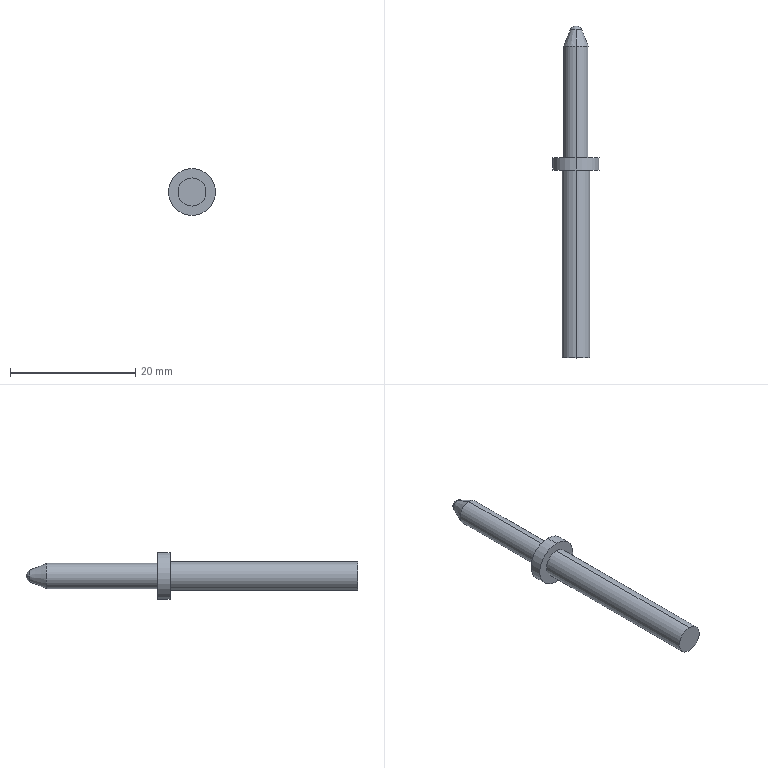Part | SolidWorks | features ICE 3, Revolution 2, Extrusion 1, RefAxis 1, RevCut 1 | 1 solid | 13 faces | box 7.5 x 53 x 7.5 mm | volume 808.158 mm3 | cylinder 6 | plane 3 | cone 2 | sphere 2 | commonest cylinder face diameters 4 x2 4.5 x2 7.5 x2
STEP:
#1=CARTESIAN_POINT('',(0.9239,20.383,0.));
#2=VERTEX_POINT('',#1);
#3=CARTESIAN_POINT('',(0.,20.383,0.9239));
#4=VERTEX_POINT('',#3);
#5=CARTESIAN_POINT('',(0.,20.383,0.));
#6=DIRECTION('',(0.,-1.,0.));
#7=DIRECTION('',(0.,0.,-1.));
#8=AXIS2_PLACEMENT_3D('',#5,#6,#7);
#9=CIRCLE('',#8,0.9239);
#10=EDGE_CURVE('',#2,#4,#9,.T.);
#11=ORIENTED_EDGE('',*,*,#10,.T.);
#12=CARTESIAN_POINT('',(0.,17.785,2.));
#13=VERTEX_POINT('',#12);
#14=CARTESIAN_POINT('',(0.,20.,1.082));
#15=DIRECTION('',(0.,-0.9239,0.3827));
#16=VECTOR('',#15,1000.);
#17=LINE('',#14,#16);
#18=EDGE_CURVE('',#4,#13,#17,.T.);
#19=ORIENTED_EDGE('',*,*,#18,.T.);
#20=CARTESIAN_POINT('',(0.,17.785,-2.));
#21=VERTEX_POINT('',#20);
#22=CARTESIAN_POINT('',(0.,17.785,0.));
#23=DIRECTION('',(0.,-1.,0.));
#24=DIRECTION('',(0.,0.,-1.));
#25=AXIS2_PLACEMENT_3D('',#22,#23,#24);
#26=CIRCLE('',#25,2.);
#27=EDGE_CURVE('',#21,#13,#26,.T.);
#28=ORIENTED_EDGE('',*,*,#27,.F.);
#29=CARTESIAN_POINT('',(0.,20.383,-0.9239));
#30=VERTEX_POINT('',#29);
#31=CARTESIAN_POINT('',(0.,20.,-1.082));
#32=DIRECTION('',(0.,-0.9239,-0.3827));
#33=VECTOR('',#32,1000.);
#34=LINE('',#31,#33);
#35=EDGE_CURVE('',#30,#21,#34,.T.);
#36=ORIENTED_EDGE('',*,*,#35,.F.);
#37=CARTESIAN_POINT('',(0.,20.383,0.));
#38=DIRECTION('',(0.,-1.,0.));
#39=DIRECTION('',(0.,0.,-1.));
#40=AXIS2_PLACEMENT_3D('',#37,#38,#39);
#41=CIRCLE('',#40,0.9239);
#42=EDGE_CURVE('',#30,#2,#41,.T.);
#43=ORIENTED_EDGE('',*,*,#42,.T.);
#44=EDGE_LOOP('',(#11,#19,#28,#36,#43));
#45=FACE_OUTER_BOUND('',#44,.T.);
#46=CARTESIAN_POINT('',(0.,20.,0.));
#47=DIRECTION('',(0.,-1.,0.));
#48=DIRECTION('',(0.,0.,-1.));
#49=AXIS2_PLACEMENT_3D('',#46,#47,#48);
#50=CONICAL_SURFACE('',#49,1.082,0.3927);
#51=ADVANCED_FACE('',(#45),#50,.T.);
#52=CARTESIAN_POINT('',(0.,21.,0.));
#53=VERTEX_POINT('',#52);
#54=CARTESIAN_POINT('',(0.,20.,0.));
#55=DIRECTION('',(0.,0.,-1.));
#56=DIRECTION('',(-1.,0.,0.));
#57=AXIS2_PLACEMENT_3D('',#54,#55,#56);
#58=CIRCLE('',#57,1.);
#59=EDGE_CURVE('',#53,#2,#58,.T.);
#60=ORIENTED_EDGE('',*,*,#59,.F.);
#61=CARTESIAN_POINT('',(-0.9239,20.383,0.));
#62=VERTEX_POINT('',#61);
#63=CARTESIAN_POINT('',(0.,20.,0.));
#64=DIRECTION('',(0.,0.,1.));
#65=DIRECTION('',(1.,0.,0.));
#66=AXIS2_PLACEMENT_3D('',#63,#64,#65);
#67=CIRCLE('',#66,1.);
#68=EDGE_CURVE('',#53,#62,#67,.T.);
#69=ORIENTED_EDGE('',*,*,#68,.T.);
#70=CARTESIAN_POINT('',(0.,20.383,0.));
#71=DIRECTION('',(0.,-1.,0.));
#72=DIRECTION('',(0.,0.,-1.));
#73=AXIS2_PLACEMENT_3D('',#70,#71,#72);
#74=CIRCLE('',#73,0.9239);
#75=EDGE_CURVE('',#4,#62,#74,.T.);
#76=ORIENTED_EDGE('',*,*,#75,.F.);
#77=ORIENTED_EDGE('',*,*,#10,.F.);
#78=EDGE_LOOP('',(#60,#69,#76,#77));
#79=FACE_OUTER_BOUND('',#78,.T.);
#80=CARTESIAN_POINT('',(0.,20.,0.));
#81=DIRECTION('',(0.,0.,1.));
#82=DIRECTION('',(1.,0.,0.));
#83=AXIS2_PLACEMENT_3D('',#80,#81,#82);
#84=SPHERICAL_SURFACE('',#83,1.);
#85=ADVANCED_FACE('',(#79),#84,.T.);
#86=ORIENTED_EDGE('',*,*,#27,.T.);
#87=CARTESIAN_POINT('',(0.,0.,2.));
#88=VERTEX_POINT('',#87);
#89=CARTESIAN_POINT('',(0.,21.,2.));
#90=DIRECTION('',(0.,-1.,0.));
#91=VECTOR('',#90,1000.);
#92=LINE('',#89,#91);
#93=EDGE_CURVE('',#13,#88,#92,.T.);
#94=ORIENTED_EDGE('',*,*,#93,.T.);
#95=CARTESIAN_POINT('',(0.,0.,-2.));
#96=VERTEX_POINT('',#95);
#97=CARTESIAN_POINT('',(0.,0.,0.));
#98=DIRECTION('',(0.,1.,0.));
#99=DIRECTION('',(0.,0.,1.));
#100=AXIS2_PLACEMENT_3D('',#97,#98,#99);
#101=CIRCLE('',#100,2.);
#102=EDGE_CURVE('',#88,#96,#101,.T.);
#103=ORIENTED_EDGE('',*,*,#102,.T.);
#104=CARTESIAN_POINT('',(0.,21.,-2.));
#105=DIRECTION('',(0.,-1.,0.));
#106=VECTOR('',#105,1000.);
#107=LINE('',#104,#106);
#108=EDGE_CURVE('',#21,#96,#107,.T.);
#109=ORIENTED_EDGE('',*,*,#108,.F.);
#110=EDGE_LOOP('',(#86,#94,#103,#109));
#111=FACE_OUTER_BOUND('',#110,.T.);
#112=CARTESIAN_POINT('',(0.,21.,0.));
#113=DIRECTION('',(0.,-1.,0.));
#114=DIRECTION('',(0.,0.,-1.));
#115=AXIS2_PLACEMENT_3D('',#112,#113,#114);
#116=CYLINDRICAL_SURFACE('',#115,2.);
#117=ADVANCED_FACE('',(#111),#116,.T.);
#118=CARTESIAN_POINT('',(0.,-32.,-2.25));
#119=VERTEX_POINT('',#118);
#120=CARTESIAN_POINT('',(0.,-32.,2.25));
#121=VERTEX_POINT('',#120);
#122=CARTESIAN_POINT('',(0.,-32.,0.));
#123=DIRECTION('',(0.,-1.,0.));
#124=DIRECTION('',(0.,0.,-1.));
#125=AXIS2_PLACEMENT_3D('',#122,#123,#124);
#126=CIRCLE('',#125,2.25);
#127=EDGE_CURVE('',#119,#121,#126,.T.);
#128=ORIENTED_EDGE('',*,*,#127,.F.);
#129=CARTESIAN_POINT('',(0.,-2.,-2.25));
#130=VERTEX_POINT('',#129);
#131=CARTESIAN_POINT('',(0.,-32.,-2.25));
#132=DIRECTION('',(0.,1.,0.));
#133=VECTOR('',#132,1000.);
#134=LINE('',#131,#133);
#135=EDGE_CURVE('',#119,#130,#134,.T.);
#136=ORIENTED_EDGE('',*,*,#135,.T.);
#137=CARTESIAN_POINT('',(0.,-2.,2.25));
#138=VERTEX_POINT('',#137);
#139=CARTESIAN_POINT('',(0.,-2.,0.));
#140=DIRECTION('',(0.,-1.,0.));
#141=DIRECTION('',(0.,0.,-1.));
#142=AXIS2_PLACEMENT_3D('',#139,#140,#141);
#143=CIRCLE('',#142,2.25);
#144=EDGE_CURVE('',#130,#138,#143,.T.);
#145=ORIENTED_EDGE('',*,*,#144,.T.);
#146=CARTESIAN_POINT('',(0.,-32.,2.25));
#147=DIRECTION('',(0.,1.,0.));
#148=VECTOR('',#147,1000.);
#149=LINE('',#146,#148);
#150=EDGE_CURVE('',#121,#138,#149,.T.);
#151=ORIENTED_EDGE('',*,*,#150,.F.);
#152=EDGE_LOOP('',(#128,#136,#145,#151));
#153=FACE_OUTER_BOUND('',#152,.T.);
#154=CARTESIAN_POINT('',(0.,-32.,0.));
#155=DIRECTION('',(0.,1.,0.));
#156=DIRECTION('',(0.,0.,1.));
#157=AXIS2_PLACEMENT_3D('',#154,#155,#156);
#158=CYLINDRICAL_SURFACE('',#157,2.25);
#159=ADVANCED_FACE('',(#153),#158,.T.);
#160=CARTESIAN_POINT('',(0.,-2.,-3.75));
#161=VERTEX_POINT('',#160);
#162=CARTESIAN_POINT('',(0.,-2.,3.75));
#163=VERTEX_POINT('',#162);
#164=CARTESIAN_POINT('',(0.,-2.,0.));
#165=DIRECTION('',(0.,-1.,0.));
#166=DIRECTION('',(0.,0.,-1.));
#167=AXIS2_PLACEMENT_3D('',#164,#165,#166);
#168=CIRCLE('',#167,3.75);
#169=EDGE_CURVE('',#161,#163,#168,.T.);
#170=ORIENTED_EDGE('',*,*,#169,.F.);
#171=CARTESIAN_POINT('',(0.,0.,-3.75));
#172=VERTEX_POINT('',#171);
#173=CARTESIAN_POINT('',(0.,-2.,-3.75));
#174=DIRECTION('',(0.,1.,0.));
#175=VECTOR('',#174,1000.);
#176=LINE('',#173,#175);
#177=EDGE_CURVE('',#161,#172,#176,.T.);
#178=ORIENTED_EDGE('',*,*,#177,.T.);
#179=CARTESIAN_POINT('',(0.,0.,3.75));
#180=VERTEX_POINT('',#179);
#181=CARTESIAN_POINT('',(0.,0.,0.));
#182=DIRECTION('',(0.,-1.,0.));
#183=DIRECTION('',(0.,0.,-1.));
#184=AXIS2_PLACEMENT_3D('',#181,#182,#183);
#185=CIRCLE('',#184,3.75);
#186=EDGE_CURVE('',#172,#180,#185,.T.);
#187=ORIENTED_EDGE('',*,*,#186,.T.);
#188=CARTESIAN_POINT('',(0.,-2.,3.75));
#189=DIRECTION('',(0.,1.,0.));
#190=VECTOR('',#189,1000.);
#191=LINE('',#188,#190);
#192=EDGE_CURVE('',#163,#180,#191,.T.);
#193=ORIENTED_EDGE('',*,*,#192,.F.);
#194=EDGE_LOOP('',(#170,#178,#187,#193));
#195=FACE_OUTER_BOUND('',#194,.T.);
#196=CARTESIAN_POINT('',(0.,-2.,0.));
#197=DIRECTION('',(0.,1.,0.));
#198=DIRECTION('',(0.,0.,1.));
#199=AXIS2_PLACEMENT_3D('',#196,#197,#198);
#200=CYLINDRICAL_SURFACE('',#199,3.75);
#201=ADVANCED_FACE('',(#195),#200,.T.);
#202=CARTESIAN_POINT('',(0.,-2.,0.));
#203=DIRECTION('',(0.,-1.,0.));
#204=DIRECTION('',(0.,0.,-1.));
#205=AXIS2_PLACEMENT_3D('',#202,#203,#204);
#206=CIRCLE('',#205,3.75);
#207=EDGE_CURVE('',#163,#161,#206,.T.);
#208=ORIENTED_EDGE('',*,*,#207,.T.);
#209=ORIENTED_EDGE('',*,*,#169,.T.);
#210=EDGE_LOOP('',(#208,#209));
#211=FACE_OUTER_BOUND('',#210,.T.);
#212=CARTESIAN_POINT('',(0.,-2.,0.));
#213=DIRECTION('',(0.,-1.,0.));
#214=DIRECTION('',(0.,0.,-1.));
#215=AXIS2_PLACEMENT_3D('',#212,#213,#214);
#216=CIRCLE('',#215,2.25);
#217=EDGE_CURVE('',#138,#130,#216,.T.);
#218=ORIENTED_EDGE('',*,*,#217,.F.);
#219=ORIENTED_EDGE('',*,*,#144,.F.);
#220=EDGE_LOOP('',(#218,#219));
#221=FACE_BOUND('',#220,.T.);
#222=CARTESIAN_POINT('',(0.,-2.,0.));
#223=DIRECTION('',(0.,-1.,0.));
#224=DIRECTION('',(0.,0.,-1.));
#225=AXIS2_PLACEMENT_3D('',#222,#223,#224);
#226=PLANE('',#225);
#227=ADVANCED_FACE('',(#211,#221),#226,.T.);
#228=CARTESIAN_POINT('',(0.,0.,0.));
#229=DIRECTION('',(0.,-1.,0.));
#230=DIRECTION('',(0.,0.,-1.));
#231=AXIS2_PLACEMENT_3D('',#228,#229,#230);
#232=CIRCLE('',#231,3.75);
#233=EDGE_CURVE('',#180,#172,#232,.T.);
#234=ORIENTED_EDGE('',*,*,#233,.F.);
#235=ORIENTED_EDGE('',*,*,#186,.F.);
#236=EDGE_LOOP('',(#234,#235));
#237=FACE_OUTER_BOUND('',#236,.T.);
#238=CARTESIAN_POINT('',(0.,0.,0.));
#239=DIRECTION('',(0.,1.,0.));
#240=DIRECTION('',(0.,0.,1.));
#241=AXIS2_PLACEMENT_3D('',#238,#239,#240);
#242=CIRCLE('',#241,2.);
#243=EDGE_CURVE('',#96,#88,#242,.T.);
#244=ORIENTED_EDGE('',*,*,#243,.F.);
#245=ORIENTED_EDGE('',*,*,#102,.F.);
#246=EDGE_LOOP('',(#244,#245));
#247=FACE_BOUND('',#246,.T.);
#248=CARTESIAN_POINT('',(0.,0.,0.));
#249=DIRECTION('',(0.,-1.,0.));
#250=DIRECTION('',(0.,0.,-1.));
#251=AXIS2_PLACEMENT_3D('',#248,#249,#250);
#252=PLANE('',#251);
#253=ADVANCED_FACE('',(#237,#247),#252,.F.);
#254=ORIENTED_EDGE('',*,*,#177,.F.);
#255=ORIENTED_EDGE('',*,*,#207,.F.);
#256=ORIENTED_EDGE('',*,*,#192,.T.);
#257=ORIENTED_EDGE('',*,*,#233,.T.);
#258=EDGE_LOOP('',(#254,#255,#256,#257));
#259=FACE_OUTER_BOUND('',#258,.T.);
#260=CARTESIAN_POINT('',(0.,-2.,0.));
#261=DIRECTION('',(0.,1.,0.));
#262=DIRECTION('',(0.,0.,1.));
#263=AXIS2_PLACEMENT_3D('',#260,#261,#262);
#264=CYLINDRICAL_SURFACE('',#263,3.75);
#265=ADVANCED_FACE('',(#259),#264,.T.);
#266=ORIENTED_EDGE('',*,*,#135,.F.);
#267=CARTESIAN_POINT('',(0.,-32.,0.));
#268=DIRECTION('',(0.,-1.,0.));
#269=DIRECTION('',(0.,0.,-1.));
#270=AXIS2_PLACEMENT_3D('',#267,#268,#269);
#271=CIRCLE('',#270,2.25);
#272=EDGE_CURVE('',#121,#119,#271,.T.);
#273=ORIENTED_EDGE('',*,*,#272,.F.);
#274=ORIENTED_EDGE('',*,*,#150,.T.);
#275=ORIENTED_EDGE('',*,*,#217,.T.);
#276=EDGE_LOOP('',(#266,#273,#274,#275));
#277=FACE_OUTER_BOUND('',#276,.T.);
#278=CARTESIAN_POINT('',(0.,-32.,0.));
#279=DIRECTION('',(0.,1.,0.));
#280=DIRECTION('',(0.,0.,1.));
#281=AXIS2_PLACEMENT_3D('',#278,#279,#280);
#282=CYLINDRICAL_SURFACE('',#281,2.25);
#283=ADVANCED_FACE('',(#277),#282,.T.);
#284=ORIENTED_EDGE('',*,*,#272,.T.);
#285=ORIENTED_EDGE('',*,*,#127,.T.);
#286=EDGE_LOOP('',(#284,#285));
#287=FACE_OUTER_BOUND('',#286,.T.);
#288=CARTESIAN_POINT('',(0.,-32.,0.));
#289=DIRECTION('',(0.,-1.,0.));
#290=DIRECTION('',(0.,0.,-1.));
#291=AXIS2_PLACEMENT_3D('',#288,#289,#290);
#292=PLANE('',#291);
#293=ADVANCED_FACE('',(#287),#292,.T.);
#294=ORIENTED_EDGE('',*,*,#93,.F.);
#295=CARTESIAN_POINT('',(0.,17.785,0.));
#296=DIRECTION('',(0.,-1.,0.));
#297=DIRECTION('',(0.,0.,-1.));
#298=AXIS2_PLACEMENT_3D('',#295,#296,#297);
#299=CIRCLE('',#298,2.);
#300=EDGE_CURVE('',#13,#21,#299,.T.);
#301=ORIENTED_EDGE('',*,*,#300,.T.);
#302=ORIENTED_EDGE('',*,*,#108,.T.);
#303=ORIENTED_EDGE('',*,*,#243,.T.);
#304=EDGE_LOOP('',(#294,#301,#302,#303));
#305=FACE_OUTER_BOUND('',#304,.T.);
#306=CARTESIAN_POINT('',(0.,21.,0.));
#307=DIRECTION('',(0.,-1.,0.));
#308=DIRECTION('',(0.,0.,-1.));
#309=AXIS2_PLACEMENT_3D('',#306,#307,#308);
#310=CYLINDRICAL_SURFACE('',#309,2.);
#311=ADVANCED_FACE('',(#305),#310,.T.);
#312=ORIENTED_EDGE('',*,*,#68,.F.);
#313=ORIENTED_EDGE('',*,*,#59,.T.);
#314=ORIENTED_EDGE('',*,*,#42,.F.);
#315=CARTESIAN_POINT('',(0.,20.383,0.));
#316=DIRECTION('',(0.,-1.,0.));
#317=DIRECTION('',(0.,0.,-1.));
#318=AXIS2_PLACEMENT_3D('',#315,#316,#317);
#319=CIRCLE('',#318,0.9239);
#320=EDGE_CURVE('',#62,#30,#319,.T.);
#321=ORIENTED_EDGE('',*,*,#320,.F.);
#322=EDGE_LOOP('',(#312,#313,#314,#321));
#323=FACE_OUTER_BOUND('',#322,.T.);
#324=CARTESIAN_POINT('',(0.,20.,0.));
#325=DIRECTION('',(0.,0.,1.));
#326=DIRECTION('',(1.,0.,0.));
#327=AXIS2_PLACEMENT_3D('',#324,#325,#326);
#328=SPHERICAL_SURFACE('',#327,1.);
#329=ADVANCED_FACE('',(#323),#328,.T.);
#330=ORIENTED_EDGE('',*,*,#18,.F.);
#331=ORIENTED_EDGE('',*,*,#75,.T.);
#332=ORIENTED_EDGE('',*,*,#320,.T.);
#333=ORIENTED_EDGE('',*,*,#35,.T.);
#334=ORIENTED_EDGE('',*,*,#300,.F.);
#335=EDGE_LOOP('',(#330,#331,#332,#333,#334));
#336=FACE_OUTER_BOUND('',#335,.T.);
#337=CARTESIAN_POINT('',(0.,20.,0.));
#338=DIRECTION('',(0.,-1.,0.));
#339=DIRECTION('',(0.,0.,-1.));
#340=AXIS2_PLACEMENT_3D('',#337,#338,#339);
#341=CONICAL_SURFACE('',#340,1.082,0.3927);
#342=ADVANCED_FACE('',(#336),#341,.T.);
#343=CLOSED_SHELL('',(#51,#85,#117,#159,#201,#227,#253,#265,#283,#293,#311,#329,#342));
#344=MANIFOLD_SOLID_BREP('',#343);
#345=CARTESIAN_POINT('',(0.,0.,0.));
#346=DIRECTION('',(0.,0.,1.));
#347=DIRECTION('',(1.,0.,0.));
#348=AXIS2_PLACEMENT_3D('',#345,#346,#347);
#349=(LENGTH_UNIT()NAMED_UNIT(*)SI_UNIT(.MILLI.,.METRE.));
#350=UNCERTAINTY_MEASURE_WITH_UNIT(LENGTH_MEASURE(0.00001),#349,'','');
#351=(NAMED_UNIT(*)PLANE_ANGLE_UNIT()SI_UNIT($,.RADIAN.));
#352=(NAMED_UNIT(*)SI_UNIT($,.STERADIAN.)SOLID_ANGLE_UNIT());
#353=(GEOMETRIC_REPRESENTATION_CONTEXT(3)GLOBAL_UNCERTAINTY_ASSIGNED_CONTEXT((#350))GLOBAL_UNIT_ASSIGNED_CONTEXT((#349,#351,#352))REPRESENTATION_CONTEXT('',''));
#354=ADVANCED_BREP_SHAPE_REPRESENTATION('',(#344,#348),#353);